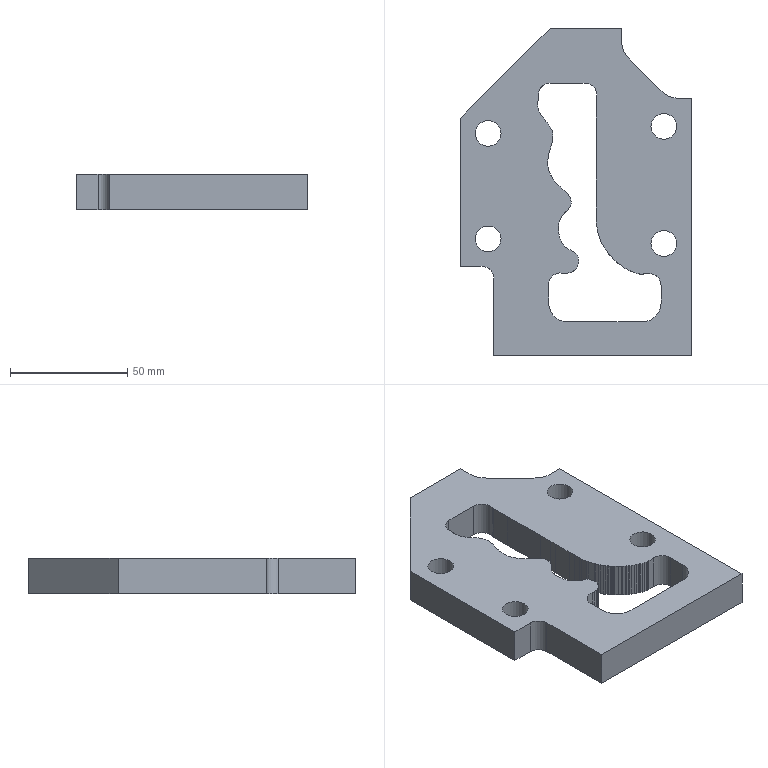Part | STEP file | 1 solid | 196 faces | box 99 x 140 x 15 mm | volume 135777 mm3 | plane 180 | cylinder 16 | commonest cylinder face diameters 10 x5 11 x4 8 x3 16 x2 20 x2